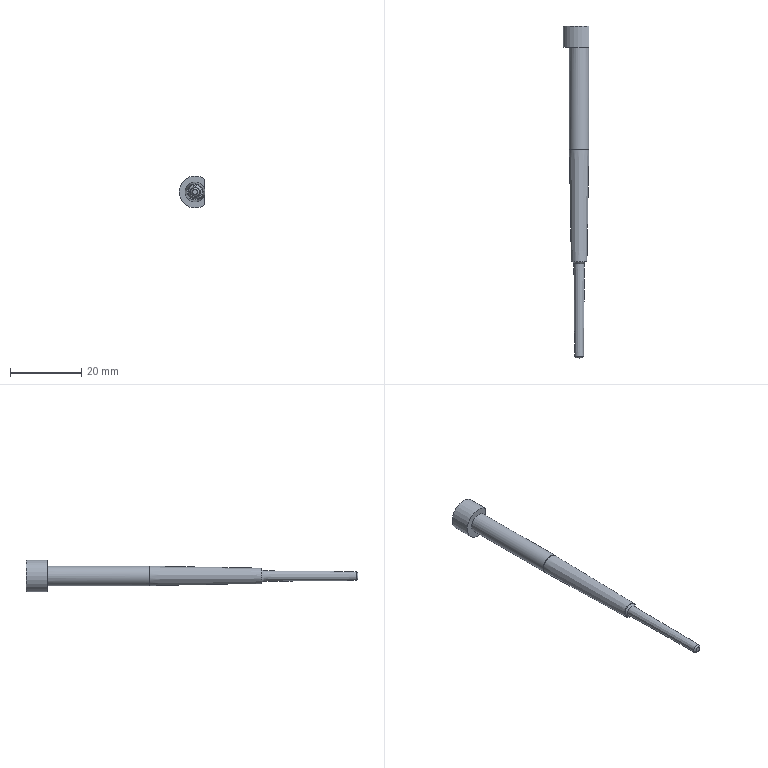Part | STEP file | solid 185 | 1 solid | 12 faces | box 7.25 x 93.183 x 8.999 mm | volume 1776 mm3 | plane 6 | cone 3 | cylinder 2 | spline 1 | commonest cylinder face diameters 5.499 x1 8.999 x1